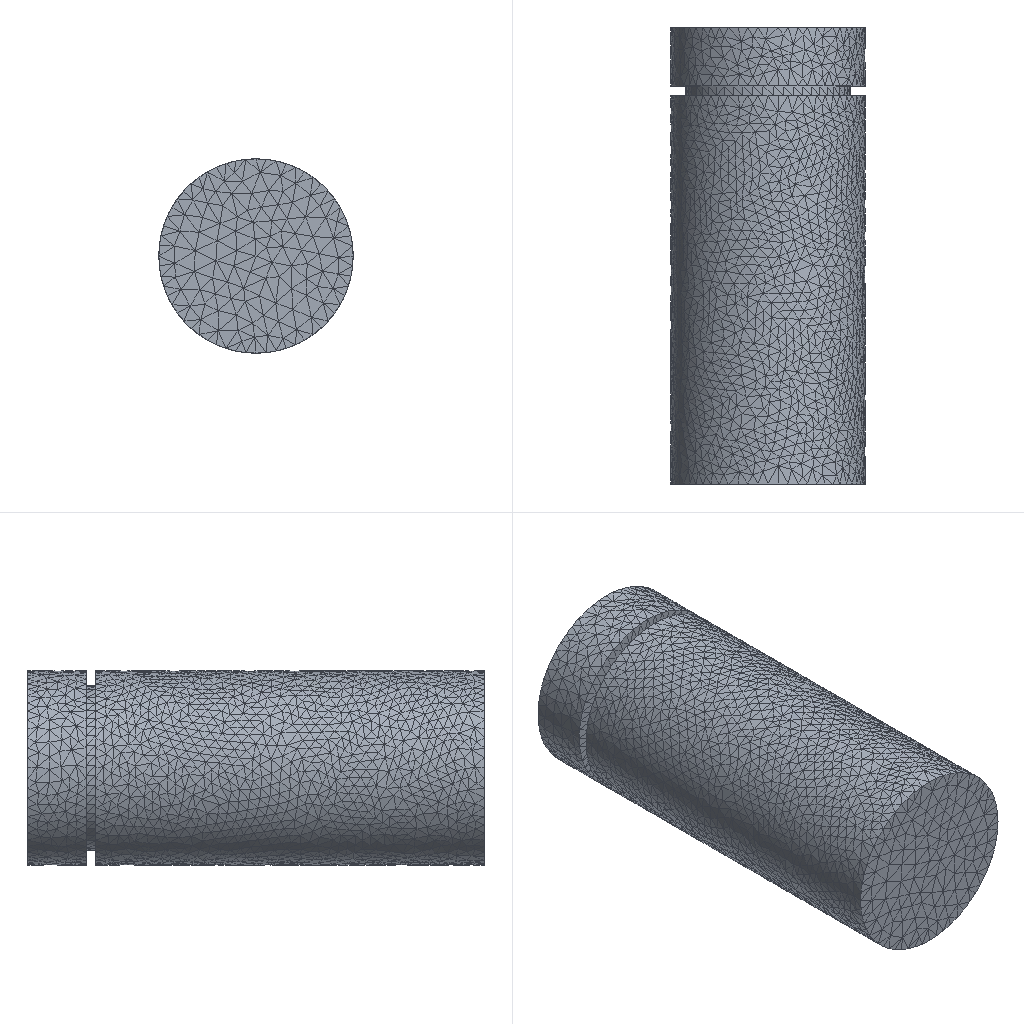Simulation study | ansys workbench
Set-up summary:
category,name,step,type,value,unit,region
solver,ansys_workbench
units,mm-N-s-tonne (MPa),,stated,"/units,MPA"
analysis,LS1,,steady-state thermal
load_step,LS1,LS1,steady-state thermal,nsubst=1; time=1
mesh,nodes,,,30932
mesh,elements,,,24219
element_type,SOLID291,,,18569
element_type,SURF152,,,5650
material,123,,conductivity,650,tonne mm s^-3 C^-1
load,Define Uniform Initial temperature,model,body load temp,22,,all
load,"Create ""Convection""",LS1,convection,0.65,,SURF152 #2
bc,,LS1,temperature,100 [dofs=TEMP],,node list
named_set,_CM32,,node,561
Ansys APDL input file, long lists of numbers shortened:
/batch
/config,noeldb,1     ! force off writing results to database
*get,_wallstrt,active,,time,wall
! ANSYS input file written by Workbench version 2023 R1
! File used for geometry attach:
/title,beike--Steady-State Thermal (A5)
! ****** Begin Custom Load Command Snippet ******
/COM, ACT Extensions:
/COM,     LSDYNA, 2023.1
/COM,/COM,     ANSYSMotion, 2023.1
/COM,
! ****** End   Custom Load Command Snippet ******
*DIM,_wb_ProjectScratch_dir,string,248
_wb_ProjectScratch_dir(1) = ''
*DIM,_wb_SolverFiles_dir,string,248
_wb_SolverFiles_dir(1) = ''
*DIM,_wb_userfiles_dir,string,248
_wb_userfiles_dir(1) = ''
/com,--- Data in consistent NMM units. See Solving Units in the help system for more information.
/units,MPA
/nopr
/wb,file,start              !  signify a WB generated input file
/prep7
! Turn off shape checking because checks already performed inside WB mesher.
! See help system for more information.
SHPP,OFF,,NOWARN
/nolist
etcon,set             ! allow ANSYS to choose best KEYOP's for 180x elements, resets any applicable keyopt to MAPDL defaults
/com,*********** Nodes for the whole assembly ***********
nblock,3,,34025
(1i9,3e20.9e3)
        1     5.000000000E+01    -3.000000000E+01    -5.000000000E+01
! (30931 more lines like these left out)
-1
/wb,elem,start            !  set before creation of elements
/com,*********** Elements for Body 1 "Solid" ***********
et,1,291
eblock,19,solid,,18569
(19i9)
        1        1        1        1        0        0        0        0       10        0        1     3883     4707     3973     4310    27317    27939    27308    27315
! (37137 more lines like these left out)
-1
/wb,elem,end               !  done creating elements
/com,*********** Send User Defined Coordinate System(s) ***********
csys,0
toffst,273.15,  ! Temperature offset from absolute zero
/wb,mat,start              !  starting to send materials
/com,*********** Send Materials ***********
MP,KXX,1,650,	! tonne mm s^-3 C^-1
/wb,mat,end                !  done sending materials
!************************* Model Summary ********************
!Solid,	123,	matid,	1
!************************* End Model Summary ********************
! get the diagonal of the bounding box. Needed later for other things
*get,_xmin,node,,mnloc,x
*get,_ymin,node,,mnloc,y
*get,_zmin,node,,mnloc,z
*get,_xmax,node,,mxloc,x
*get,_ymax,node,,mxloc,y
*get,_zmax,node,,mxloc,z
_ASMDIAG=(_xmax-_xmin)*(_xmax-_xmin)+(_ymax-_ymin)*(_ymax-_ymin)+(_zmax-_zmin)*(_zmax-_zmin)
_ASMDIAG=SQRT(_ASMDIAG)
/wb,contact,start          !  starting to send contact
/wb,contact,end            !  done creating contacts
/golist
/wb,load,start             !  starting to send loads
/com,*********** Define Temperature Constraint ***********
CMBLOCK,_CM32   ,NODE,      561
(8i10)
       223       224       225       226       227       228       229       230
! (70 more lines like these left out)
fcum,add                   ! add nodal forces up (needed in case have loads on the same edge,vertex)
fcum                       ! reset default on fcum command since done sending WB F loads
/com,*********** Create "Convection" ***********
et,2,152
eblock,10,,,5650
(15i9)
    24470        2        2        2        0      172      171      599      599     5965     5966      599     5971
! (5649 more lines like these left out)
-1
esel,s,type,,2
keyop,2,8,2.
keyop,2,13,0
esel,all
/com,***************** Define Uniform Initial temperature ***************
tunif,22.
/gst,on,on
fini
*get,_numnode,node,0,count
*get,_numelem,elem,0,count
*get, _MAXELEMNUM, elem, 0, NUM, MAX
*get, _MAXNODENUM, node, 0, NUM, MAX
*get, _MAXELEMTYPE, etyp, 0, NUM, MAX
*get, _MAXREALCONST, rcon, 0, NUM, MAX
/go
/wb,load,end               !  done creating loads
/com,--- Number of total nodes = %_numnode%
/com,--- Number of contact elements = 5650
/com,--- Number of spring elements = 0
/com,--- Number of bearing elements = 0
/com,--- Number of solid elements = 18569
/com,--- Number of condensed parts = 0
/com,--- Number of total elements = %_numelem%
*get,_wallbsol,active,,time,wall
/com,****************************************************************************
/com,*************************    SOLUTION       ********************************
/com,****************************************************************************
/solu
antype,0                   ! static analysis
!eqsl,sparse               ! using sparse solver which is default so no eqsl command needed
cntr,print,1               ! print out contact info and also make no initial contact an error
rescontrol,,none                 ! Do not keep any restart files
dmpoption,emat,no             ! Don't combine emat file for DANSYS
dmpoption,esav,no             ! Don't combine esav file for DANSYS
/com,****************************************************
/com,******************* SOLVE FOR LS 1 OF 1 ****************
d,_CM32,temp,100.
esel,s,type,,2
nsle
sf,all,conv,0.65,22.
nsel,all
esel,all
/nopr
/gopr
autots,on
nsub,1,10,1
time,1.
outres,erase
outres,all,none
outres,nsol,all
outres,rsol,all
outres,eangl,all
outres,veng,all
outres,fflux,all
outres,cont,all
/nopr
esel,s,type,,2
cm,_elmisc,elem
esel,all
/gopr
outres,misc,all,_elmisc
cnvtol,heat,,.001,,1.e-003    ! Program Controlled. Set MINREF equivalent of 1e-6 Watts
! *********** WB SOLVE COMMAND ***********
! check interactive state
*get,ANSINTER_,active,,int
*if,ANSINTER_,ne,0,then
/eof
*endif
solve
/com *************** Write FE CONNECTORS *********
CEWRITE,file,ce,,INTE
/com,****************************************************
/com,*************** FINISHED SOLVE FOR LS 1 *************
*get,_wallasol,active,,time,wall
/post1
xmlo,ENCODING,ISO-8859-1
xmlo,parm
/xml,parm,xml
fini
/gopr
*get,_walldone,active,,time,wall
_preptime=(_wallbsol-_wallstrt)*3600
_solvtime=(_wallasol-_wallbsol)*3600
_posttime=(_walldone-_wallasol)*3600
_totaltim=(_walldone-_wallstrt)*3600
*get,_dlbratio,active,0,solu,dlbr
*get,_combtime,active,0,solu,comb
*get,_ssmode,active,0,solu,ssmm
*get,_ndofs,active,0,solu,ndof
/fclean				!clean distributed files
/com,--- Total number of nodes = %_numnode%
/com,--- Total number of elements = %_numelem%
/com,--- Element load balance ratio = %_dlbratio%
/com,--- Time to combine distributed files = %_combtime%
/com,--- Sparse memory mode = %_ssmode%
/com,--- Number of DOF = %_ndofs%
/wb,file,end               ! done with WB generated input
Results summary:
result,analyses[0].index,,,1
result,analyses[0].system,,,SYS
result,analyses[0].deck,,,deck.dat
result,analyses[0].solve_status,,,completed
result,analyses[0].analysis_type,,,static
result,analyses[0].physics,,,thermal
result,analyses[0].unit_system,,,"NMM: mm, ton, N, s, mV, mA, degC"
result,analyses[0].n_sets,,,1
result,analyses[0].load_steps[0].set,set=1,,1
result,analyses[0].load_steps[0].time_or_freq,set=1,,1
result,analyses[0].load_steps[0].max_temperature,set=1,,100
result,analyses[0].load_steps[0].min_temperature,set=1,,49.39
result,geometry_export[0][0],,,.step
result,geometry_export[0][1],,,ok
result,geometry_export[0][2],,,1